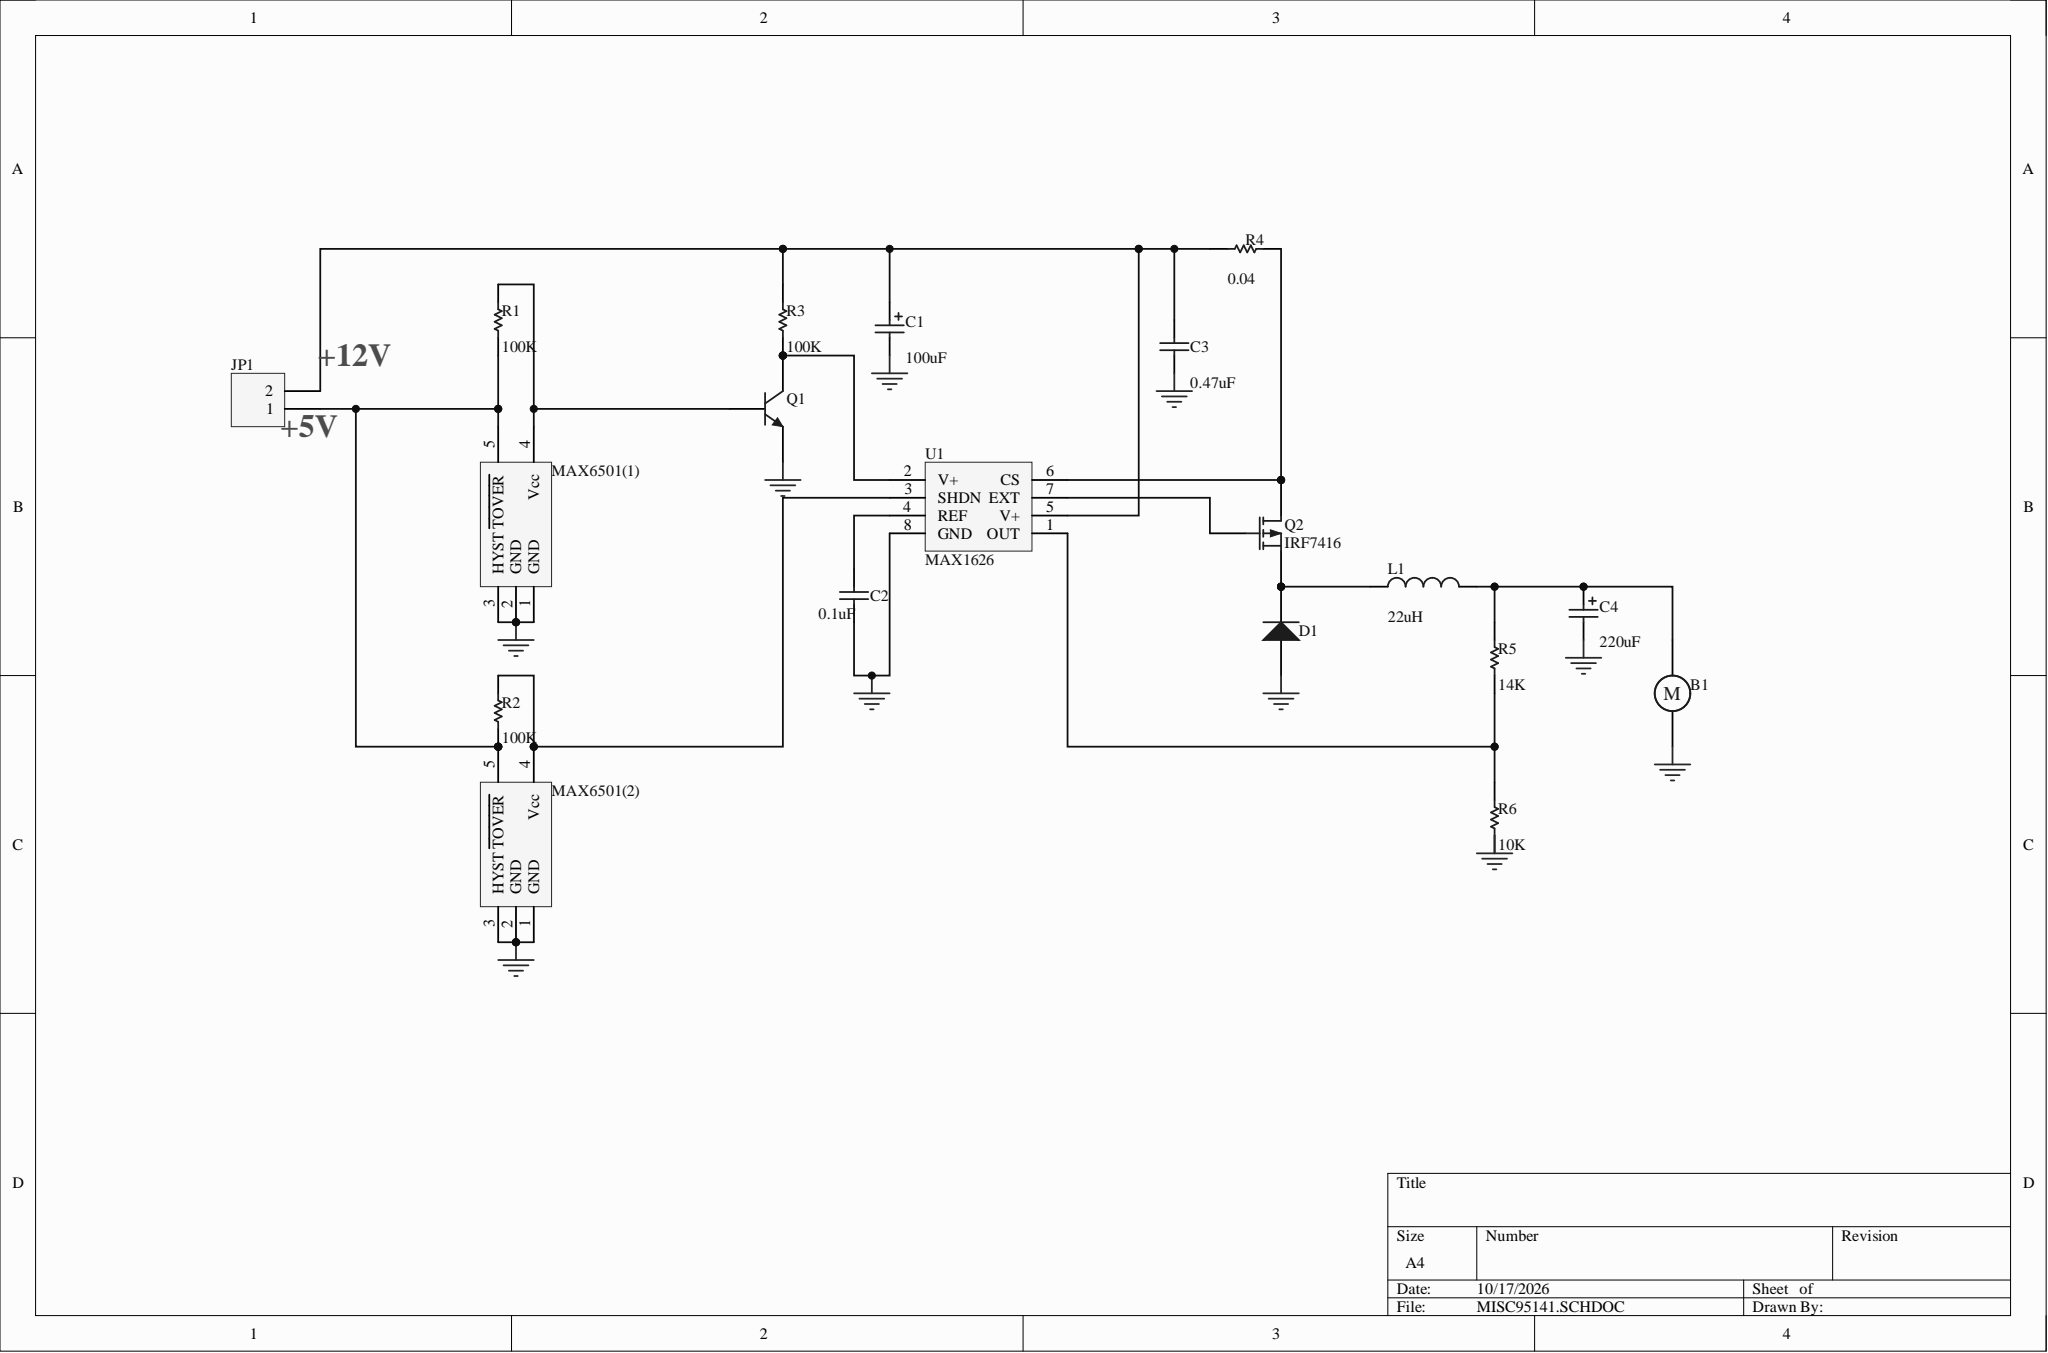Circuit board | Cadence Allegro | 19 parts | 12 nets
Bill of materials:
Comment,Description,Designator,Footprint,LibRef,Quantity
"Motor","Motor, General Kind","B1","RB5-10.5","Motor","1"
"Cap Pol1","Polarized Capacitor (Radial)","C1, C4","RB7.6-15","Cap Pol1","2"
"Cap","Capacitor","C2, C3","RAD-0.3","Cap","2"
"Diode","Default Diode","D1","DSO-C2/X3.3","Diode","1"
"Header 2","Header, 2-Pin","JP1","HDR1X2","Header 2","1"
"Inductor","Inductor","L1","CC4532-1812","Inductor","1"
"MAX6501","","MAX6501(1), MAX6501(2)","SO-G5/P.95","MAX6501","2"
"NPN","NPN Bipolar Transistor","Q1","BCY-W3","NPN","1"
"IRF7416","P-Channel MOSFET","Q2","BCY-W3/H.8","MOSFET-P","1"
"Res1","Resistor","R1, R2, R3, R4, R5, R6","AXIAL-0.3","Res1","6"
"MAX1626","","U1","DIP-4","MAX1626","1"
Netlist (Protel format):
[
B1
RB5-10.5
Motor



]
[
C1
RB7.6-15
Cap Pol1



]
[
C2
RAD-0.3
Cap



]
[
C3
RAD-0.3
Cap



]
[
C4
RB7.6-15
Cap Pol1



]
[
D1
DSO-C2/X3.3
Diode



]
[
JP1
HDR1X2
Header 2



]
[
L1
CC4532-1812
Inductor



]
[
MAX6501(1)
SO-G5/P.95
MAX6501



]
[
MAX6501(2)
SO-G5/P.95
MAX6501



]
[
Q1
BCY-W3
NPN



]
[
Q2
BCY-W3/H.8
IRF7416



]
[
R1
AXIAL-0.3
Res1



]
[
R2
AXIAL-0.3
Res1



]
[
R3
AXIAL-0.3
Res1



]
[
R4
AXIAL-0.3
Res1



]
[
R5
AXIAL-0.3
Res1



]
[
R6
AXIAL-0.3
Res1



]
[
U1
DIP-4
MAX1626



]
(
NetR5_1
R5-1
R6-2
U1-1
)
(
NetQ2_2
Q2-2
U1-7
)
(
NetQ2_1
Q2-1
R4-2
U1-6
)
(
NetQ1_1
Q1-1
R3-1
U1-2
)
(
NetMAX6501(2)_4
MAX6501(2)-4
R2-2
U1-3
)
(
NetMAX6501(1)_4
MAX6501(1)-4
Q1-2
R1-2
)
(
NetJP1_1
JP1-1
MAX6501(1)-5
MAX6501(2)-5
R1-1
R2-1
)
(
NetD1_2
D1-2
L1-1
Q2-3
)
(
NetC2_2
C2-2
U1-4
)
(
NetC1_1
C1-1
C3-2
JP1-2
R3-2
R4-1
U1-5
)
(
NetB1_1
B1-1
C4-1
L1-2
R5-2
)
(
GND
B1-2
C1-2
C2-1
C3-1
C4-2
D1-1
MAX6501(1)-1
MAX6501(1)-2
MAX6501(1)-3
MAX6501(2)-1
MAX6501(2)-2
MAX6501(2)-3
Q1-3
U1-8
)